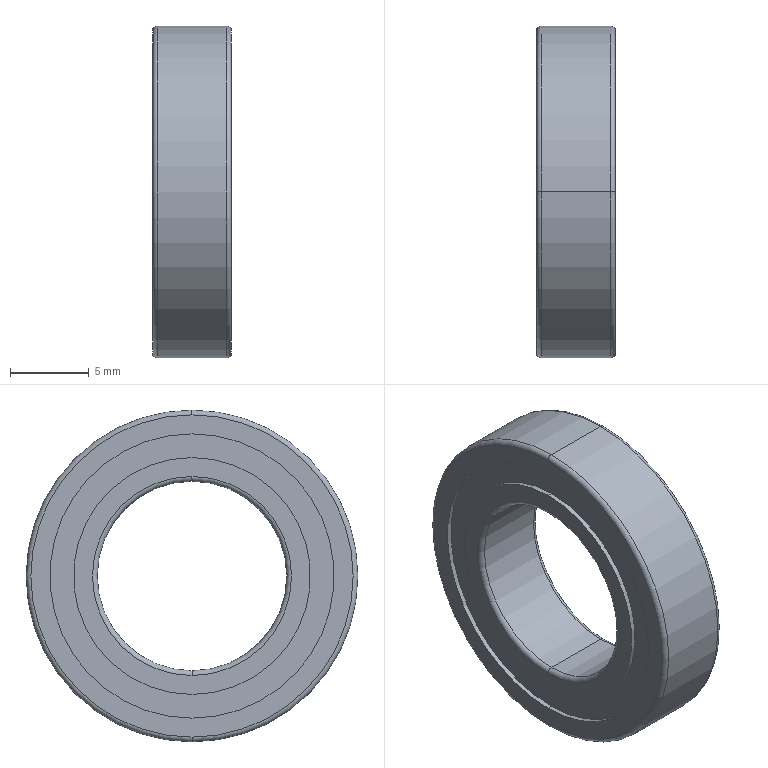Part | STEP file | 61801ZZ_Rolling bearings 61801 GB 276-94 | 1 solid | 144 faces | box 5 x 21 x 21 mm | volume 933.169 mm3 | torus 74 | sphere 42 | cylinder 20 | plane 8 | commonest cylinder face diameters 15 x8 18 x8 12 x2 21 x2